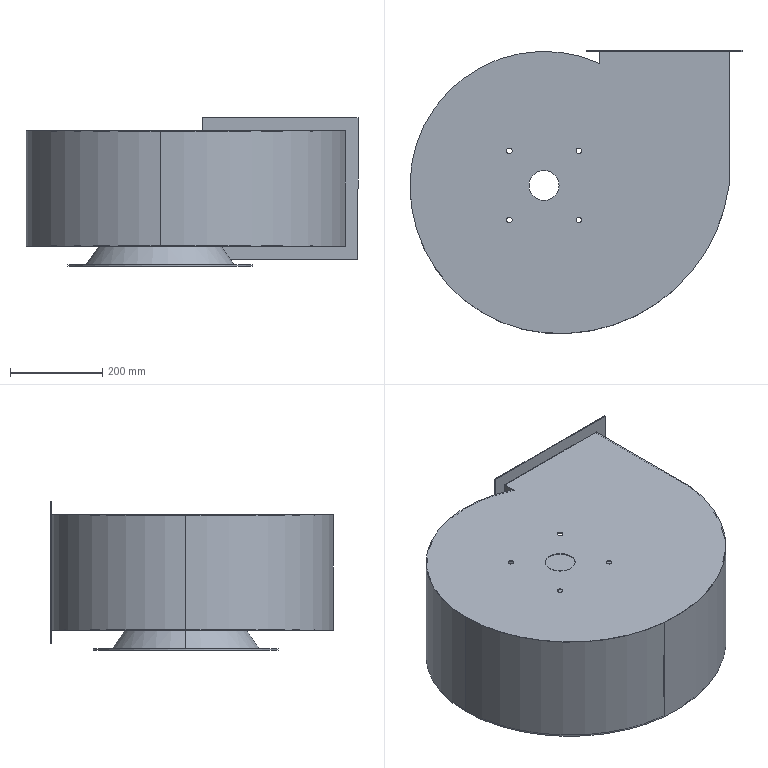Part | STEP file | Produce dryer line heating fan-SIROCCOFAN-3KW-COVER | 2 solids | 63 faces | box 718 x 612.214 x 321 mm | volume 2543268 mm3 | cylinder 38 | plane 21 | cone 4 | commonest cylinder face diameters 10 x16 12 x8 65 x2 260 x2 315 x2 400 x2